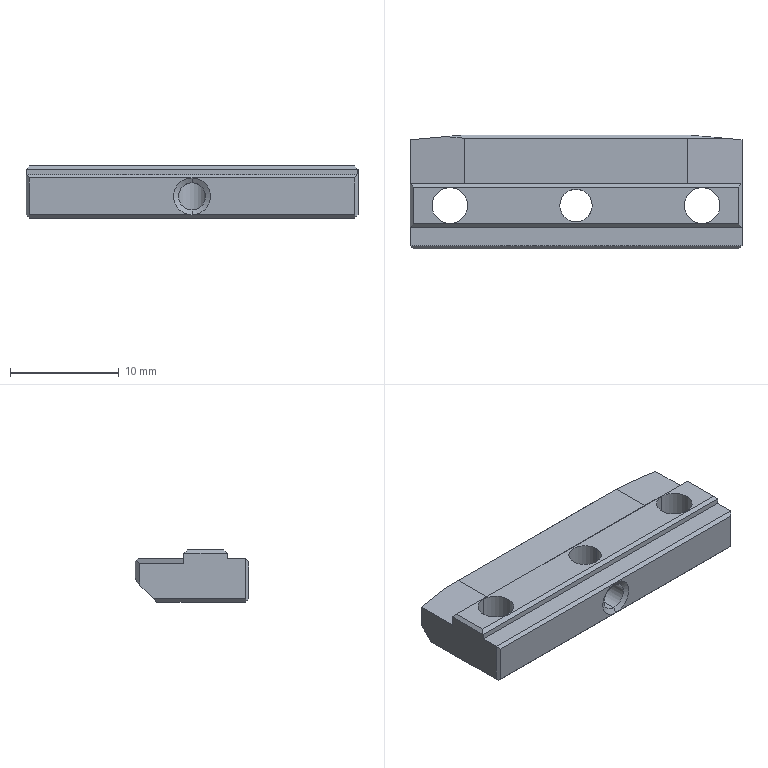Part | NX | 1 solid | 43 faces | box 30.6 x 10.5 x 4.8 mm | volume 1169 mm3 | plane 29 | cylinder 8 | cone 6 | commonest cylinder face diameters 3.3 x4 2.5 x2 3 x2